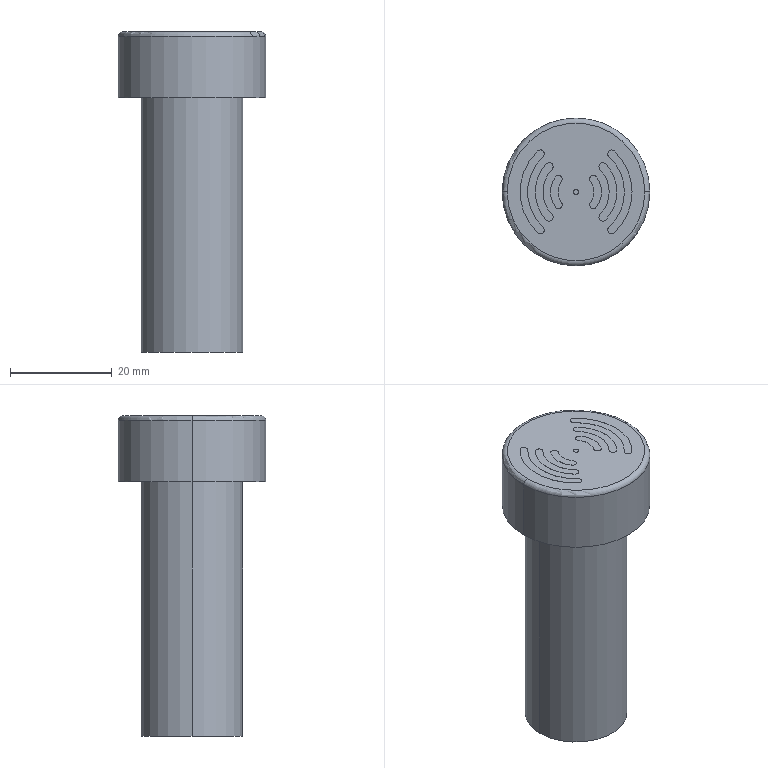Part | STEP file | Flashing buzzer AD17-SML-DC24V | 2 solids | 58 faces | box 29 x 29 x 63 mm | volume 18875 mm3 | cylinder 44 | plane 12 | torus 2 | commonest cylinder face diameters 1.5 x18 7 x3 10 x3 13 x3 16 x3 19 x3